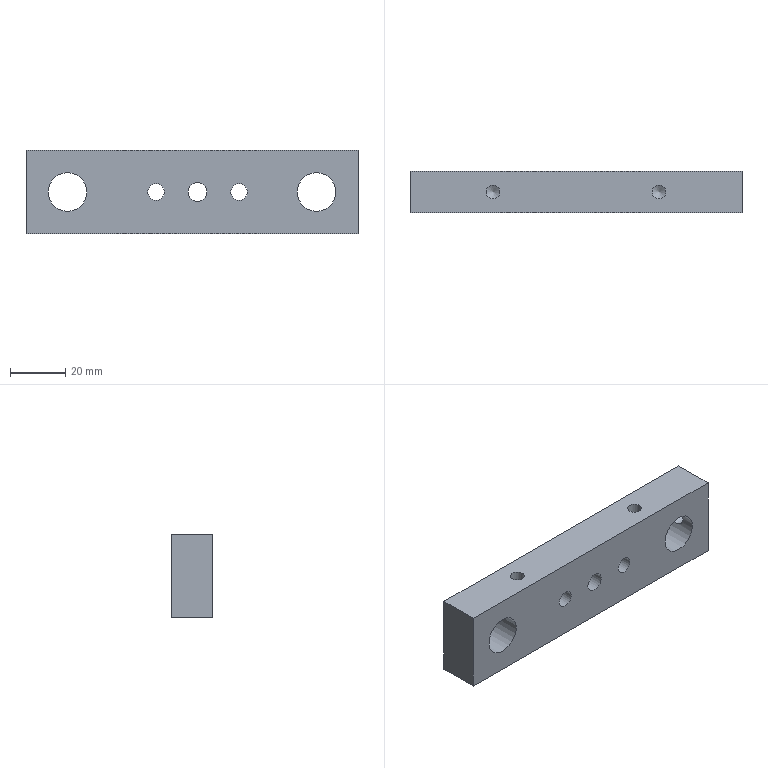Part | NX | features BREP 1 | 1 solid | 16 faces | box 120 x 15 x 30 mm | volume 47220 mm3 | cylinder 8 | plane 6 | cone 2 | commonest cylinder face diameters 5 x3 6 x2 14 x2 6.8 x1
STEP:
#1=CARTESIAN_POINT('',(60.,0.,-2.5));
#2=VERTEX_POINT('',#1);
#3=CARTESIAN_POINT('',(60.,0.,0.));
#4=DIRECTION('',(1.,0.,0.));
#5=DIRECTION('',(0.,0.,-1.));
#6=AXIS2_PLACEMENT_3D('',#3,#4,#5);
#7=CIRCLE('',#6,2.5);
#8=EDGE_CURVE('',#2,#2,#7,.T.);
#9=ORIENTED_EDGE('',*,*,#8,.F.);
#10=EDGE_LOOP('',(#9));
#11=FACE_BOUND('',#10,.T.);
#12=CARTESIAN_POINT('',(60.,-7.5,15.));
#13=VERTEX_POINT('',#12);
#14=CARTESIAN_POINT('',(60.,-7.5,-15.));
#15=VERTEX_POINT('',#14);
#16=CARTESIAN_POINT('',(60.,-7.5,15.));
#17=DIRECTION('',(0.,0.,-1.));
#18=VECTOR('',#17,1000.);
#19=LINE('',#16,#18);
#20=EDGE_CURVE('',#13,#15,#19,.T.);
#21=ORIENTED_EDGE('',*,*,#20,.T.);
#22=CARTESIAN_POINT('',(60.,7.5,-15.));
#23=VERTEX_POINT('',#22);
#24=CARTESIAN_POINT('',(60.,7.5,-15.));
#25=DIRECTION('',(0.,-1.,0.));
#26=VECTOR('',#25,1000.);
#27=LINE('',#24,#26);
#28=EDGE_CURVE('',#23,#15,#27,.T.);
#29=ORIENTED_EDGE('',*,*,#28,.F.);
#30=CARTESIAN_POINT('',(60.,7.5,15.));
#31=VERTEX_POINT('',#30);
#32=CARTESIAN_POINT('',(60.,7.5,15.));
#33=DIRECTION('',(0.,0.,-1.));
#34=VECTOR('',#33,1000.);
#35=LINE('',#32,#34);
#36=EDGE_CURVE('',#31,#23,#35,.T.);
#37=ORIENTED_EDGE('',*,*,#36,.F.);
#38=CARTESIAN_POINT('',(60.,7.5,15.));
#39=DIRECTION('',(0.,-1.,0.));
#40=VECTOR('',#39,1000.);
#41=LINE('',#38,#40);
#42=EDGE_CURVE('',#31,#13,#41,.T.);
#43=ORIENTED_EDGE('',*,*,#42,.T.);
#44=EDGE_LOOP('',(#21,#29,#37,#43));
#45=FACE_BOUND('',#44,.T.);
#46=CARTESIAN_POINT('',(60.,7.5,15.));
#47=DIRECTION('',(-1.,0.,0.));
#48=DIRECTION('',(0.,0.,-1.));
#49=AXIS2_PLACEMENT_3D('',#46,#47,#48);
#50=PLANE('',#49);
#51=ADVANCED_FACE('',(#11,#45),#50,.F.);
#52=CARTESIAN_POINT('',(-60.,-7.5,-15.));
#53=VERTEX_POINT('',#52);
#54=CARTESIAN_POINT('',(-60.,-7.5,-15.));
#55=DIRECTION('',(-1.,0.,0.));
#56=VECTOR('',#55,1000.);
#57=LINE('',#54,#56);
#58=EDGE_CURVE('',#15,#53,#57,.T.);
#59=ORIENTED_EDGE('',*,*,#58,.T.);
#60=CARTESIAN_POINT('',(-60.,7.5,-15.));
#61=VERTEX_POINT('',#60);
#62=CARTESIAN_POINT('',(-60.,7.5,-15.));
#63=DIRECTION('',(0.,-1.,0.));
#64=VECTOR('',#63,1000.);
#65=LINE('',#62,#64);
#66=EDGE_CURVE('',#61,#53,#65,.T.);
#67=ORIENTED_EDGE('',*,*,#66,.F.);
#68=CARTESIAN_POINT('',(-60.,7.5,-15.));
#69=DIRECTION('',(-1.,0.,0.));
#70=VECTOR('',#69,1000.);
#71=LINE('',#68,#70);
#72=EDGE_CURVE('',#23,#61,#71,.T.);
#73=ORIENTED_EDGE('',*,*,#72,.F.);
#74=ORIENTED_EDGE('',*,*,#28,.T.);
#75=EDGE_LOOP('',(#59,#67,#73,#74));
#76=FACE_BOUND('',#75,.T.);
#77=CARTESIAN_POINT('',(-60.,7.5,-15.));
#78=DIRECTION('',(0.,0.,1.));
#79=DIRECTION('',(-1.,0.,0.));
#80=AXIS2_PLACEMENT_3D('',#77,#78,#79);
#81=PLANE('',#80);
#82=ADVANCED_FACE('',(#76),#81,.F.);
#83=CARTESIAN_POINT('',(-60.,-7.5,15.));
#84=VERTEX_POINT('',#83);
#85=CARTESIAN_POINT('',(-60.,-7.5,15.));
#86=DIRECTION('',(0.,0.,1.));
#87=VECTOR('',#86,1000.);
#88=LINE('',#85,#87);
#89=EDGE_CURVE('',#53,#84,#88,.T.);
#90=ORIENTED_EDGE('',*,*,#89,.T.);
#91=CARTESIAN_POINT('',(-60.,7.5,15.));
#92=VERTEX_POINT('',#91);
#93=CARTESIAN_POINT('',(-60.,7.5,15.));
#94=DIRECTION('',(0.,-1.,0.));
#95=VECTOR('',#94,1000.);
#96=LINE('',#93,#95);
#97=EDGE_CURVE('',#92,#84,#96,.T.);
#98=ORIENTED_EDGE('',*,*,#97,.F.);
#99=CARTESIAN_POINT('',(-60.,7.5,15.));
#100=DIRECTION('',(0.,0.,1.));
#101=VECTOR('',#100,1000.);
#102=LINE('',#99,#101);
#103=EDGE_CURVE('',#61,#92,#102,.T.);
#104=ORIENTED_EDGE('',*,*,#103,.F.);
#105=ORIENTED_EDGE('',*,*,#66,.T.);
#106=EDGE_LOOP('',(#90,#98,#104,#105));
#107=FACE_BOUND('',#106,.T.);
#108=CARTESIAN_POINT('',(-60.,7.5,15.));
#109=DIRECTION('',(1.,0.,0.));
#110=DIRECTION('',(0.,0.,1.));
#111=AXIS2_PLACEMENT_3D('',#108,#109,#110);
#112=PLANE('',#111);
#113=ADVANCED_FACE('',(#107),#112,.F.);
#114=CARTESIAN_POINT('',(-27.5,0.,15.));
#115=VERTEX_POINT('',#114);
#116=CARTESIAN_POINT('',(-30.,0.,15.));
#117=DIRECTION('',(0.,0.,1.));
#118=DIRECTION('',(1.,0.,0.));
#119=AXIS2_PLACEMENT_3D('',#116,#117,#118);
#120=CIRCLE('',#119,2.5);
#121=EDGE_CURVE('',#115,#115,#120,.T.);
#122=ORIENTED_EDGE('',*,*,#121,.F.);
#123=EDGE_LOOP('',(#122));
#124=FACE_BOUND('',#123,.T.);
#125=CARTESIAN_POINT('',(32.5,0.,15.));
#126=VERTEX_POINT('',#125);
#127=CARTESIAN_POINT('',(30.,0.,15.));
#128=DIRECTION('',(0.,0.,1.));
#129=DIRECTION('',(1.,0.,0.));
#130=AXIS2_PLACEMENT_3D('',#127,#128,#129);
#131=CIRCLE('',#130,2.5);
#132=EDGE_CURVE('',#126,#126,#131,.T.);
#133=ORIENTED_EDGE('',*,*,#132,.F.);
#134=EDGE_LOOP('',(#133));
#135=FACE_BOUND('',#134,.T.);
#136=CARTESIAN_POINT('',(-60.,-7.5,15.));
#137=DIRECTION('',(1.,0.,0.));
#138=VECTOR('',#137,1000.);
#139=LINE('',#136,#138);
#140=EDGE_CURVE('',#84,#13,#139,.T.);
#141=ORIENTED_EDGE('',*,*,#140,.T.);
#142=ORIENTED_EDGE('',*,*,#42,.F.);
#143=CARTESIAN_POINT('',(-60.,7.5,15.));
#144=DIRECTION('',(1.,0.,0.));
#145=VECTOR('',#144,1000.);
#146=LINE('',#143,#145);
#147=EDGE_CURVE('',#92,#31,#146,.T.);
#148=ORIENTED_EDGE('',*,*,#147,.F.);
#149=ORIENTED_EDGE('',*,*,#97,.T.);
#150=EDGE_LOOP('',(#141,#142,#148,#149));
#151=FACE_BOUND('',#150,.T.);
#152=CARTESIAN_POINT('',(-60.,7.5,15.));
#153=DIRECTION('',(0.,0.,-1.));
#154=DIRECTION('',(1.,0.,0.));
#155=AXIS2_PLACEMENT_3D('',#152,#153,#154);
#156=PLANE('',#155);
#157=ADVANCED_FACE('',(#124,#135,#151),#156,.F.);
#158=CARTESIAN_POINT('',(45.,7.5,7.));
#159=VERTEX_POINT('',#158);
#160=CARTESIAN_POINT('',(45.,7.5,0.));
#161=DIRECTION('',(0.,1.,0.));
#162=DIRECTION('',(0.,0.,1.));
#163=AXIS2_PLACEMENT_3D('',#160,#161,#162);
#164=CIRCLE('',#163,7.);
#165=EDGE_CURVE('',#159,#159,#164,.T.);
#166=ORIENTED_EDGE('',*,*,#165,.F.);
#167=EDGE_LOOP('',(#166));
#168=FACE_BOUND('',#167,.T.);
#169=CARTESIAN_POINT('',(-45.,7.5,7.));
#170=VERTEX_POINT('',#169);
#171=CARTESIAN_POINT('',(-45.,7.5,0.));
#172=DIRECTION('',(0.,1.,0.));
#173=DIRECTION('',(0.,0.,1.));
#174=AXIS2_PLACEMENT_3D('',#171,#172,#173);
#175=CIRCLE('',#174,7.);
#176=EDGE_CURVE('',#170,#170,#175,.T.);
#177=ORIENTED_EDGE('',*,*,#176,.F.);
#178=EDGE_LOOP('',(#177));
#179=FACE_BOUND('',#178,.T.);
#180=CARTESIAN_POINT('',(-13.,7.5,3.));
#181=VERTEX_POINT('',#180);
#182=CARTESIAN_POINT('',(-13.,7.5,0.));
#183=DIRECTION('',(0.,1.,0.));
#184=DIRECTION('',(0.,0.,1.));
#185=AXIS2_PLACEMENT_3D('',#182,#183,#184);
#186=CIRCLE('',#185,3.);
#187=EDGE_CURVE('',#181,#181,#186,.T.);
#188=ORIENTED_EDGE('',*,*,#187,.F.);
#189=EDGE_LOOP('',(#188));
#190=FACE_BOUND('',#189,.T.);
#191=CARTESIAN_POINT('',(17.,7.5,3.));
#192=VERTEX_POINT('',#191);
#193=CARTESIAN_POINT('',(17.,7.5,0.));
#194=DIRECTION('',(0.,1.,0.));
#195=DIRECTION('',(0.,0.,1.));
#196=AXIS2_PLACEMENT_3D('',#193,#194,#195);
#197=CIRCLE('',#196,3.);
#198=EDGE_CURVE('',#192,#192,#197,.T.);
#199=ORIENTED_EDGE('',*,*,#198,.F.);
#200=EDGE_LOOP('',(#199));
#201=FACE_BOUND('',#200,.T.);
#202=CARTESIAN_POINT('',(2.,7.5,3.4));
#203=VERTEX_POINT('',#202);
#204=CARTESIAN_POINT('',(2.,7.5,0.));
#205=DIRECTION('',(0.,1.,0.));
#206=DIRECTION('',(0.,0.,1.));
#207=AXIS2_PLACEMENT_3D('',#204,#205,#206);
#208=CIRCLE('',#207,3.4);
#209=EDGE_CURVE('',#203,#203,#208,.T.);
#210=ORIENTED_EDGE('',*,*,#209,.F.);
#211=EDGE_LOOP('',(#210));
#212=FACE_BOUND('',#211,.T.);
#213=ORIENTED_EDGE('',*,*,#36,.T.);
#214=ORIENTED_EDGE('',*,*,#72,.T.);
#215=ORIENTED_EDGE('',*,*,#103,.T.);
#216=ORIENTED_EDGE('',*,*,#147,.T.);
#217=EDGE_LOOP('',(#213,#214,#215,#216));
#218=FACE_BOUND('',#217,.T.);
#219=CARTESIAN_POINT('',(0.,7.5,0.));
#220=DIRECTION('',(0.,-1.,0.));
#221=DIRECTION('',(0.,0.,1.));
#222=AXIS2_PLACEMENT_3D('',#219,#220,#221);
#223=PLANE('',#222);
#224=ADVANCED_FACE('',(#168,#179,#190,#201,#212,#218),#223,.F.);
#225=CARTESIAN_POINT('',(45.,-7.5,7.));
#226=VERTEX_POINT('',#225);
#227=CARTESIAN_POINT('',(45.,-7.5,0.));
#228=DIRECTION('',(0.,1.,0.));
#229=DIRECTION('',(0.,0.,1.));
#230=AXIS2_PLACEMENT_3D('',#227,#228,#229);
#231=CIRCLE('',#230,7.);
#232=EDGE_CURVE('',#226,#226,#231,.T.);
#233=ORIENTED_EDGE('',*,*,#232,.T.);
#234=EDGE_LOOP('',(#233));
#235=FACE_BOUND('',#234,.T.);
#236=CARTESIAN_POINT('',(-45.,-7.5,7.));
#237=VERTEX_POINT('',#236);
#238=CARTESIAN_POINT('',(-45.,-7.5,0.));
#239=DIRECTION('',(0.,1.,0.));
#240=DIRECTION('',(0.,0.,1.));
#241=AXIS2_PLACEMENT_3D('',#238,#239,#240);
#242=CIRCLE('',#241,7.);
#243=EDGE_CURVE('',#237,#237,#242,.T.);
#244=ORIENTED_EDGE('',*,*,#243,.T.);
#245=EDGE_LOOP('',(#244));
#246=FACE_BOUND('',#245,.T.);
#247=CARTESIAN_POINT('',(-13.,-7.5,3.));
#248=VERTEX_POINT('',#247);
#249=CARTESIAN_POINT('',(-13.,-7.5,0.));
#250=DIRECTION('',(0.,1.,0.));
#251=DIRECTION('',(0.,0.,1.));
#252=AXIS2_PLACEMENT_3D('',#249,#250,#251);
#253=CIRCLE('',#252,3.);
#254=EDGE_CURVE('',#248,#248,#253,.T.);
#255=ORIENTED_EDGE('',*,*,#254,.T.);
#256=EDGE_LOOP('',(#255));
#257=FACE_BOUND('',#256,.T.);
#258=CARTESIAN_POINT('',(17.,-7.5,3.));
#259=VERTEX_POINT('',#258);
#260=CARTESIAN_POINT('',(17.,-7.5,0.));
#261=DIRECTION('',(0.,1.,0.));
#262=DIRECTION('',(0.,0.,1.));
#263=AXIS2_PLACEMENT_3D('',#260,#261,#262);
#264=CIRCLE('',#263,3.);
#265=EDGE_CURVE('',#259,#259,#264,.T.);
#266=ORIENTED_EDGE('',*,*,#265,.T.);
#267=EDGE_LOOP('',(#266));
#268=FACE_BOUND('',#267,.T.);
#269=CARTESIAN_POINT('',(2.,-7.5,3.4));
#270=VERTEX_POINT('',#269);
#271=CARTESIAN_POINT('',(2.,-7.5,0.));
#272=DIRECTION('',(0.,1.,0.));
#273=DIRECTION('',(0.,0.,1.));
#274=AXIS2_PLACEMENT_3D('',#271,#272,#273);
#275=CIRCLE('',#274,3.4);
#276=EDGE_CURVE('',#270,#270,#275,.T.);
#277=ORIENTED_EDGE('',*,*,#276,.T.);
#278=EDGE_LOOP('',(#277));
#279=FACE_BOUND('',#278,.T.);
#280=ORIENTED_EDGE('',*,*,#20,.F.);
#281=ORIENTED_EDGE('',*,*,#140,.F.);
#282=ORIENTED_EDGE('',*,*,#89,.F.);
#283=ORIENTED_EDGE('',*,*,#58,.F.);
#284=EDGE_LOOP('',(#280,#281,#282,#283));
#285=FACE_BOUND('',#284,.T.);
#286=CARTESIAN_POINT('',(0.,-7.5,0.));
#287=DIRECTION('',(0.,-1.,0.));
#288=DIRECTION('',(0.,0.,1.));
#289=AXIS2_PLACEMENT_3D('',#286,#287,#288);
#290=PLANE('',#289);
#291=ADVANCED_FACE('',(#235,#246,#257,#268,#279,#285),#290,.T.);
#292=ORIENTED_EDGE('',*,*,#276,.F.);
#293=EDGE_LOOP('',(#292));
#294=FACE_BOUND('',#293,.T.);
#295=ORIENTED_EDGE('',*,*,#209,.T.);
#296=EDGE_LOOP('',(#295));
#297=FACE_BOUND('',#296,.T.);
#298=CARTESIAN_POINT('',(2.,7.5,0.));
#299=DIRECTION('',(0.,1.,0.));
#300=DIRECTION('',(0.,0.,-1.));
#301=AXIS2_PLACEMENT_3D('',#298,#299,#300);
#302=CYLINDRICAL_SURFACE('',#301,3.4);
#303=ADVANCED_FACE('',(#294,#297),#302,.F.);
#304=ORIENTED_EDGE('',*,*,#265,.F.);
#305=EDGE_LOOP('',(#304));
#306=FACE_BOUND('',#305,.T.);
#307=ORIENTED_EDGE('',*,*,#198,.T.);
#308=EDGE_LOOP('',(#307));
#309=FACE_BOUND('',#308,.T.);
#310=CARTESIAN_POINT('',(17.,7.5,0.));
#311=DIRECTION('',(0.,1.,0.));
#312=DIRECTION('',(0.,0.,-1.));
#313=AXIS2_PLACEMENT_3D('',#310,#311,#312);
#314=CYLINDRICAL_SURFACE('',#313,3.);
#315=ADVANCED_FACE('',(#306,#309),#314,.F.);
#316=ORIENTED_EDGE('',*,*,#254,.F.);
#317=EDGE_LOOP('',(#316));
#318=FACE_BOUND('',#317,.T.);
#319=ORIENTED_EDGE('',*,*,#187,.T.);
#320=EDGE_LOOP('',(#319));
#321=FACE_BOUND('',#320,.T.);
#322=CARTESIAN_POINT('',(-13.,7.5,0.));
#323=DIRECTION('',(0.,1.,0.));
#324=DIRECTION('',(0.,0.,-1.));
#325=AXIS2_PLACEMENT_3D('',#322,#323,#324);
#326=CYLINDRICAL_SURFACE('',#325,3.);
#327=ADVANCED_FACE('',(#318,#321),#326,.F.);
#328=ORIENTED_EDGE('',*,*,#243,.F.);
#329=EDGE_LOOP('',(#328));
#330=FACE_BOUND('',#329,.T.);
#331=ORIENTED_EDGE('',*,*,#176,.T.);
#332=EDGE_LOOP('',(#331));
#333=FACE_BOUND('',#332,.T.);
#334=CARTESIAN_POINT('',(-45.,7.5,0.));
#335=DIRECTION('',(0.,1.,0.));
#336=DIRECTION('',(0.,0.,-1.));
#337=AXIS2_PLACEMENT_3D('',#334,#335,#336);
#338=CYLINDRICAL_SURFACE('',#337,7.);
#339=ADVANCED_FACE('',(#330,#333),#338,.F.);
#340=CARTESIAN_POINT('',(51.538,0.,-2.5));
#341=VERTEX_POINT('',#340);
#342=CARTESIAN_POINT('',(51.777,-1.958,-1.96));
#343=CARTESIAN_POINT('',(51.419,-0.0002842,-2.771));
#344=CARTESIAN_POINT('',(51.777,1.959,-1.958));
#345=CARTESIAN_POINT('',(52.112,2.771,-0.003326));
#346=CARTESIAN_POINT('',(51.777,1.957,1.961));
#347=CARTESIAN_POINT('',(51.419,0.001892,2.77));
#348=CARTESIAN_POINT('',(51.777,-1.959,1.96));
#349=CARTESIAN_POINT('',(52.112,-2.771,-0.000483));
#350=CARTESIAN_POINT('',(51.777,-1.958,-1.96));
#351=CARTESIAN_POINT('',(51.419,-0.0002842,-2.771));
#352=CARTESIAN_POINT('',(51.777,1.959,-1.958));
#353=B_SPLINE_CURVE_WITH_KNOTS('',3,(#342,#343,#344,#345,#346,#347,#348,#349,#350,#351,#352),.UNSPECIFIED.,.T.,.F.,(1,1,1,1,1,1,1,1,1,1,1,1,1,1,1),(-0.00591,-0.00394,-0.00197,0.,0.00197,0.00394,0.00591,0.007881,0.009851,0.01182,0.01379,0.01576,0.01773,0.0197,0.02167),.UNSPECIFIED.);
#354=EDGE_CURVE('',#341,#341,#353,.T.);
#355=ORIENTED_EDGE('',*,*,#354,.T.);
#356=EDGE_LOOP('',(#355));
#357=FACE_BOUND('',#356,.T.);
#358=ORIENTED_EDGE('',*,*,#232,.F.);
#359=EDGE_LOOP('',(#358));
#360=FACE_BOUND('',#359,.T.);
#361=ORIENTED_EDGE('',*,*,#165,.T.);
#362=EDGE_LOOP('',(#361));
#363=FACE_BOUND('',#362,.T.);
#364=CARTESIAN_POINT('',(45.,7.5,0.));
#365=DIRECTION('',(0.,1.,0.));
#366=DIRECTION('',(0.,0.,-1.));
#367=AXIS2_PLACEMENT_3D('',#364,#365,#366);
#368=CYLINDRICAL_SURFACE('',#367,7.);
#369=ADVANCED_FACE('',(#357,#360,#363),#368,.F.);
#370=CARTESIAN_POINT('',(30.,0.,-1.502));
#371=VERTEX_POINT('',#370);
#372=VERTEX_LOOP('',#371);
#373=FACE_BOUND('',#372,.T.);
#374=CARTESIAN_POINT('',(32.5,0.,0.));
#375=VERTEX_POINT('',#374);
#376=CARTESIAN_POINT('',(30.,0.,0.));
#377=DIRECTION('',(0.,0.,1.));
#378=DIRECTION('',(1.,0.,0.));
#379=AXIS2_PLACEMENT_3D('',#376,#377,#378);
#380=CIRCLE('',#379,2.5);
#381=EDGE_CURVE('',#375,#375,#380,.T.);
#382=ORIENTED_EDGE('',*,*,#381,.T.);
#383=EDGE_LOOP('',(#382));
#384=FACE_BOUND('',#383,.T.);
#385=CARTESIAN_POINT('',(30.,0.,0.));
#386=DIRECTION('',(0.,0.,1.));
#387=DIRECTION('',(-1.,0.,0.));
#388=AXIS2_PLACEMENT_3D('',#385,#386,#387);
#389=CONICAL_SURFACE('',#388,2.5,1.03);
#390=ADVANCED_FACE('',(#373,#384),#389,.F.);
#391=ORIENTED_EDGE('',*,*,#381,.F.);
#392=EDGE_LOOP('',(#391));
#393=FACE_BOUND('',#392,.T.);
#394=ORIENTED_EDGE('',*,*,#132,.T.);
#395=EDGE_LOOP('',(#394));
#396=FACE_BOUND('',#395,.T.);
#397=CARTESIAN_POINT('',(30.,0.,15.));
#398=DIRECTION('',(0.,0.,1.));
#399=DIRECTION('',(-1.,0.,0.));
#400=AXIS2_PLACEMENT_3D('',#397,#398,#399);
#401=CYLINDRICAL_SURFACE('',#400,2.5);
#402=ADVANCED_FACE('',(#393,#396),#401,.F.);
#403=CARTESIAN_POINT('',(-30.,0.,-1.502));
#404=VERTEX_POINT('',#403);
#405=VERTEX_LOOP('',#404);
#406=FACE_BOUND('',#405,.T.);
#407=CARTESIAN_POINT('',(-27.5,0.,0.));
#408=VERTEX_POINT('',#407);
#409=CARTESIAN_POINT('',(-30.,0.,0.));
#410=DIRECTION('',(0.,0.,1.));
#411=DIRECTION('',(1.,0.,0.));
#412=AXIS2_PLACEMENT_3D('',#409,#410,#411);
#413=CIRCLE('',#412,2.5);
#414=EDGE_CURVE('',#408,#408,#413,.T.);
#415=ORIENTED_EDGE('',*,*,#414,.T.);
#416=EDGE_LOOP('',(#415));
#417=FACE_BOUND('',#416,.T.);
#418=CARTESIAN_POINT('',(-30.,0.,0.));
#419=DIRECTION('',(0.,0.,1.));
#420=DIRECTION('',(-1.,0.,0.));
#421=AXIS2_PLACEMENT_3D('',#418,#419,#420);
#422=CONICAL_SURFACE('',#421,2.5,1.03);
#423=ADVANCED_FACE('',(#406,#417),#422,.F.);
#424=ORIENTED_EDGE('',*,*,#414,.F.);
#425=EDGE_LOOP('',(#424));
#426=FACE_BOUND('',#425,.T.);
#427=ORIENTED_EDGE('',*,*,#121,.T.);
#428=EDGE_LOOP('',(#427));
#429=FACE_BOUND('',#428,.T.);
#430=CARTESIAN_POINT('',(-30.,0.,15.));
#431=DIRECTION('',(0.,0.,1.));
#432=DIRECTION('',(-1.,0.,0.));
#433=AXIS2_PLACEMENT_3D('',#430,#431,#432);
#434=CYLINDRICAL_SURFACE('',#433,2.5);
#435=ADVANCED_FACE('',(#426,#429),#434,.F.);
#436=ORIENTED_EDGE('',*,*,#8,.T.);
#437=EDGE_LOOP('',(#436));
#438=FACE_BOUND('',#437,.T.);
#439=ORIENTED_EDGE('',*,*,#354,.F.);
#440=EDGE_LOOP('',(#439));
#441=FACE_BOUND('',#440,.T.);
#442=CARTESIAN_POINT('',(60.,0.,0.));
#443=DIRECTION('',(1.,0.,0.));
#444=DIRECTION('',(0.,0.,1.));
#445=AXIS2_PLACEMENT_3D('',#442,#443,#444);
#446=CYLINDRICAL_SURFACE('',#445,2.5);
#447=ADVANCED_FACE('',(#438,#441),#446,.F.);
#448=CLOSED_SHELL('',(#51,#82,#113,#157,#224,#291,#303,#315,#327,#339,#369,#390,#402,#423,#435,#447));
#449=MANIFOLD_SOLID_BREP('',#448);
#450=(LENGTH_UNIT()NAMED_UNIT(*)SI_UNIT(.MILLI.,.METRE.));
#451=UNCERTAINTY_MEASURE_WITH_UNIT(LENGTH_MEASURE(0.0508),#450,'','');
#452=(NAMED_UNIT(*)PLANE_ANGLE_UNIT()SI_UNIT($,.RADIAN.));
#453=(NAMED_UNIT(*)SI_UNIT($,.STERADIAN.)SOLID_ANGLE_UNIT());
#454=(GEOMETRIC_REPRESENTATION_CONTEXT(3)GLOBAL_UNCERTAINTY_ASSIGNED_CONTEXT((#451))GLOBAL_UNIT_ASSIGNED_CONTEXT((#450,#452,#453))REPRESENTATION_CONTEXT('',''));
#455=ADVANCED_BREP_SHAPE_REPRESENTATION('',(#449),#454);